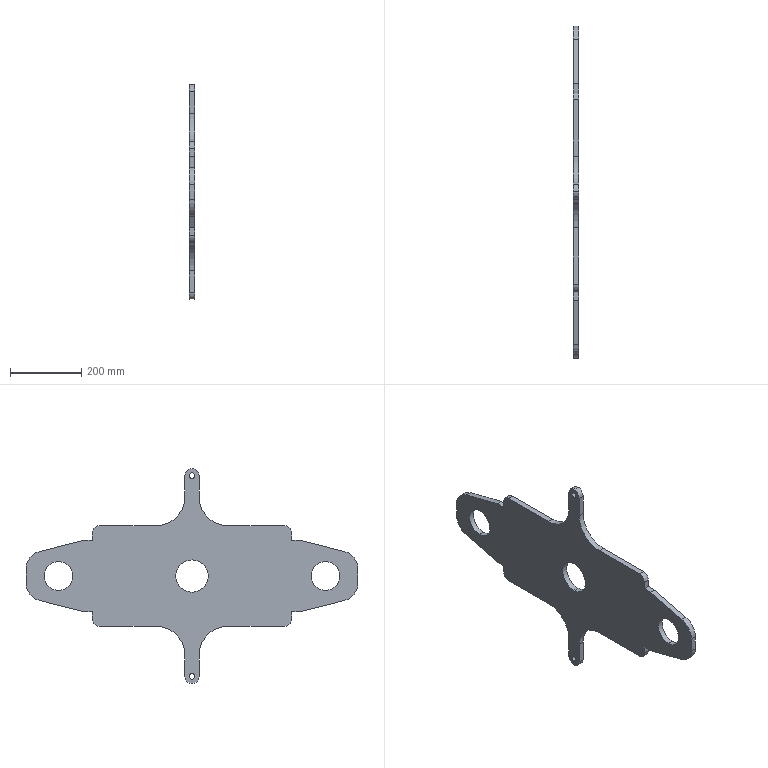Part | SolidWorks | features Extrusion 1, Fillet 1, HoleWzd 1, ICE 1 | 1 solid | 49 faces | box 16 x 930 x 602 mm | volume 3486837 mm3 | cylinder 25 | plane 24 | commonest cylinder face diameters 40 x7 16 x4 80.5 x4 100 x4 160 x4 90.5 x2